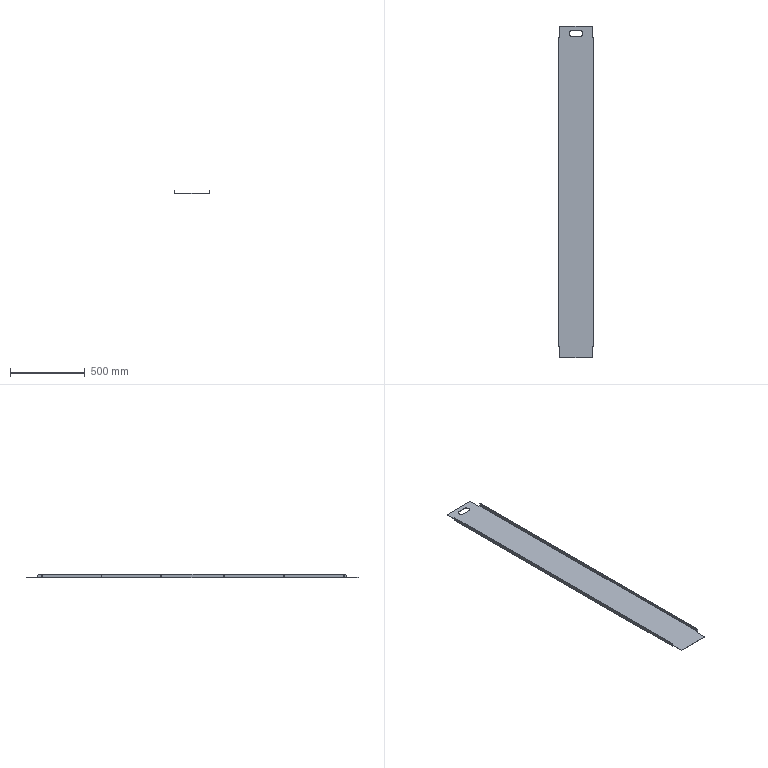Part | SolidWorks | features Chamfer 2, ICE 2, Cut 1, FlatPattern 1, SMBaseFlange 1, SheetMetal 1 | 1 solid | 65 faces | box 240 x 2216 x 23 mm | volume 917548 mm3 | plane 34 | cylinder 31 | commonest cylinder face diameters 6.2 x24 40 x3 0.4 x2 3.4 x2